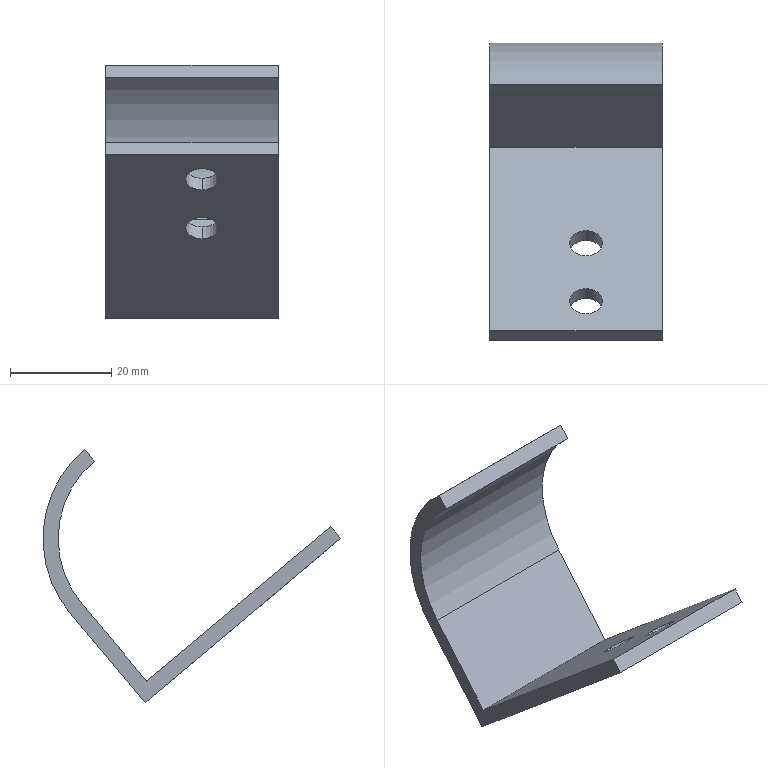Part | SolidWorks | features BaseBody 1 | 1 solid | 14 faces | box 34 x 58.835 x 50.022 mm | volume 10435 mm3 | plane 8 | cylinder 6 | commonest cylinder face diameters 6.5 x4 40 x1 46 x1
STEP:
#1=CARTESIAN_POINT('',(-85.,219.284,-334.482));
#2=VERTEX_POINT('',#1);
#3=CARTESIAN_POINT('',(-85.,224.263,-338.66));
#4=VERTEX_POINT('',#3);
#5=CARTESIAN_POINT('',(-85.,221.774,-336.571));
#6=DIRECTION('',(0.,-0.6428,-0.766));
#7=DIRECTION('',(0.,-0.766,0.6428));
#8=AXIS2_PLACEMENT_3D('',#5,#6,#7);
#9=CIRCLE('',#8,3.25);
#10=EDGE_CURVE('',#2,#4,#9,.T.);
#11=ORIENTED_EDGE('',*,*,#10,.T.);
#12=CARTESIAN_POINT('',(-85.,226.192,-336.362));
#13=VERTEX_POINT('',#12);
#14=CARTESIAN_POINT('',(-85.,219.764,-344.023));
#15=DIRECTION('',(0.,0.6428,0.766));
#16=VECTOR('',#15,1000.);
#17=LINE('',#14,#16);
#18=EDGE_CURVE('',#4,#13,#17,.T.);
#19=ORIENTED_EDGE('',*,*,#18,.T.);
#20=CARTESIAN_POINT('',(-85.,221.212,-332.184));
#21=VERTEX_POINT('',#20);
#22=CARTESIAN_POINT('',(-85.,223.702,-334.273));
#23=DIRECTION('',(0.,-0.6428,-0.766));
#24=DIRECTION('',(0.,-0.766,0.6428));
#25=AXIS2_PLACEMENT_3D('',#22,#23,#24);
#26=CIRCLE('',#25,3.25);
#27=EDGE_CURVE('',#21,#13,#26,.T.);
#28=ORIENTED_EDGE('',*,*,#27,.F.);
#29=CARTESIAN_POINT('',(-85.,214.785,-339.844));
#30=DIRECTION('',(0.,0.6428,0.766));
#31=VECTOR('',#30,1000.);
#32=LINE('',#29,#31);
#33=EDGE_CURVE('',#2,#21,#32,.T.);
#34=ORIENTED_EDGE('',*,*,#33,.F.);
#35=EDGE_LOOP('',(#11,#19,#28,#34));
#36=FACE_OUTER_BOUND('',#35,.T.);
#37=CARTESIAN_POINT('',(-85.,217.274,-341.934));
#38=DIRECTION('',(0.,0.6428,0.766));
#39=DIRECTION('',(0.,-0.766,0.6428));
#40=AXIS2_PLACEMENT_3D('',#37,#38,#39);
#41=CYLINDRICAL_SURFACE('',#40,3.25);
#42=ADVANCED_FACE('',(#36),#41,.F.);
#43=CARTESIAN_POINT('',(-85.,207.803,-324.848));
#44=VERTEX_POINT('',#43);
#45=CARTESIAN_POINT('',(-85.,212.782,-329.026));
#46=VERTEX_POINT('',#45);
#47=CARTESIAN_POINT('',(-85.,210.292,-326.937));
#48=DIRECTION('',(0.,-0.6428,-0.766));
#49=DIRECTION('',(0.,-0.766,0.6428));
#50=AXIS2_PLACEMENT_3D('',#47,#48,#49);
#51=CIRCLE('',#50,3.25);
#52=EDGE_CURVE('',#44,#46,#51,.T.);
#53=ORIENTED_EDGE('',*,*,#52,.T.);
#54=CARTESIAN_POINT('',(-85.,214.71,-326.728));
#55=VERTEX_POINT('',#54);
#56=CARTESIAN_POINT('',(-85.,208.282,-334.388));
#57=DIRECTION('',(0.,0.6428,0.766));
#58=VECTOR('',#57,1000.);
#59=LINE('',#56,#58);
#60=EDGE_CURVE('',#46,#55,#59,.T.);
#61=ORIENTED_EDGE('',*,*,#60,.T.);
#62=CARTESIAN_POINT('',(-85.,209.731,-322.55));
#63=VERTEX_POINT('',#62);
#64=CARTESIAN_POINT('',(-85.,212.221,-324.639));
#65=DIRECTION('',(0.,-0.6428,-0.766));
#66=DIRECTION('',(0.,-0.766,0.6428));
#67=AXIS2_PLACEMENT_3D('',#64,#65,#66);
#68=CIRCLE('',#67,3.25);
#69=EDGE_CURVE('',#63,#55,#68,.T.);
#70=ORIENTED_EDGE('',*,*,#69,.F.);
#71=CARTESIAN_POINT('',(-85.,203.303,-330.21));
#72=DIRECTION('',(0.,0.6428,0.766));
#73=VECTOR('',#72,1000.);
#74=LINE('',#71,#73);
#75=EDGE_CURVE('',#44,#63,#74,.T.);
#76=ORIENTED_EDGE('',*,*,#75,.F.);
#77=EDGE_LOOP('',(#53,#61,#70,#76));
#78=FACE_OUTER_BOUND('',#77,.T.);
#79=CARTESIAN_POINT('',(-85.,205.793,-332.299));
#80=DIRECTION('',(0.,0.6428,0.766));
#81=DIRECTION('',(0.,-0.766,0.6428));
#82=AXIS2_PLACEMENT_3D('',#79,#80,#81);
#83=CYLINDRICAL_SURFACE('',#82,3.25);
#84=ADVANCED_FACE('',(#78),#83,.F.);
#85=CARTESIAN_POINT('',(-104.,204.42,-322.01));
#86=VERTEX_POINT('',#85);
#87=CARTESIAN_POINT('',(-70.,204.42,-322.01));
#88=VERTEX_POINT('',#87);
#89=CARTESIAN_POINT('',(-100.,204.42,-322.01));
#90=DIRECTION('',(1.,0.,0.));
#91=VECTOR('',#90,1000.);
#92=LINE('',#89,#91);
#93=EDGE_CURVE('',#86,#88,#92,.T.);
#94=ORIENTED_EDGE('',*,*,#93,.F.);
#95=CARTESIAN_POINT('',(-104.,243.09,-354.458));
#96=VERTEX_POINT('',#95);
#97=CARTESIAN_POINT('',(-104.,243.09,-354.458));
#98=DIRECTION('',(0.,-0.766,0.6428));
#99=VECTOR('',#98,1000.);
#100=LINE('',#97,#99);
#101=EDGE_CURVE('',#96,#86,#100,.T.);
#102=ORIENTED_EDGE('',*,*,#101,.F.);
#103=CARTESIAN_POINT('',(-70.,243.09,-354.458));
#104=VERTEX_POINT('',#103);
#105=CARTESIAN_POINT('',(-100.,243.09,-354.458));
#106=DIRECTION('',(-1.,0.,0.));
#107=VECTOR('',#106,1000.);
#108=LINE('',#105,#107);
#109=EDGE_CURVE('',#104,#96,#108,.T.);
#110=ORIENTED_EDGE('',*,*,#109,.F.);
#111=CARTESIAN_POINT('',(-70.,243.09,-354.458));
#112=DIRECTION('',(0.,0.766,-0.6428));
#113=VECTOR('',#112,1000.);
#114=LINE('',#111,#113);
#115=EDGE_CURVE('',#88,#104,#114,.T.);
#116=ORIENTED_EDGE('',*,*,#115,.F.);
#117=EDGE_LOOP('',(#94,#102,#110,#116));
#118=FACE_OUTER_BOUND('',#117,.T.);
#119=ORIENTED_EDGE('',*,*,#10,.F.);
#120=CARTESIAN_POINT('',(-85.,221.774,-336.571));
#121=DIRECTION('',(0.,-0.6428,-0.766));
#122=DIRECTION('',(0.,-0.766,0.6428));
#123=AXIS2_PLACEMENT_3D('',#120,#121,#122);
#124=CIRCLE('',#123,3.25);
#125=EDGE_CURVE('',#4,#2,#124,.T.);
#126=ORIENTED_EDGE('',*,*,#125,.F.);
#127=EDGE_LOOP('',(#119,#126));
#128=FACE_BOUND('',#127,.T.);
#129=ORIENTED_EDGE('',*,*,#52,.F.);
#130=CARTESIAN_POINT('',(-85.,210.292,-326.937));
#131=DIRECTION('',(0.,-0.6428,-0.766));
#132=DIRECTION('',(0.,-0.766,0.6428));
#133=AXIS2_PLACEMENT_3D('',#130,#131,#132);
#134=CIRCLE('',#133,3.25);
#135=EDGE_CURVE('',#46,#44,#134,.T.);
#136=ORIENTED_EDGE('',*,*,#135,.F.);
#137=EDGE_LOOP('',(#129,#136));
#138=FACE_BOUND('',#137,.T.);
#139=CARTESIAN_POINT('',(-100.,243.09,-354.458));
#140=DIRECTION('',(0.,0.6428,0.766));
#141=DIRECTION('',(0.,-0.766,0.6428));
#142=AXIS2_PLACEMENT_3D('',#139,#140,#141);
#143=PLANE('',#142);
#144=ADVANCED_FACE('',(#118,#128,#138),#143,.F.);
#145=CARTESIAN_POINT('',(-70.,255.039,-304.436));
#146=VERTEX_POINT('',#145);
#147=CARTESIAN_POINT('',(-70.,253.111,-306.734));
#148=VERTEX_POINT('',#147);
#149=CARTESIAN_POINT('',(-70.,255.039,-304.436));
#150=DIRECTION('',(0.,-0.6428,-0.766));
#151=VECTOR('',#150,1000.);
#152=LINE('',#149,#151);
#153=EDGE_CURVE('',#146,#148,#152,.T.);
#154=ORIENTED_EDGE('',*,*,#153,.T.);
#155=CARTESIAN_POINT('',(-70.,255.576,-334.91));
#156=VERTEX_POINT('',#155);
#157=CARTESIAN_POINT('',(-70.,240.255,-322.055));
#158=DIRECTION('',(-1.,0.,0.));
#159=DIRECTION('',(0.,0.,-1.));
#160=AXIS2_PLACEMENT_3D('',#157,#158,#159);
#161=CIRCLE('',#160,20.);
#162=EDGE_CURVE('',#148,#156,#161,.T.);
#163=ORIENTED_EDGE('',*,*,#162,.T.);
#164=CARTESIAN_POINT('',(-70.,242.72,-350.231));
#165=VERTEX_POINT('',#164);
#166=CARTESIAN_POINT('',(-70.,255.576,-334.91));
#167=DIRECTION('',(0.,-0.6428,-0.766));
#168=VECTOR('',#167,1000.);
#169=LINE('',#166,#168);
#170=EDGE_CURVE('',#156,#165,#169,.T.);
#171=ORIENTED_EDGE('',*,*,#170,.T.);
#172=CARTESIAN_POINT('',(-70.,206.349,-319.712));
#173=VERTEX_POINT('',#172);
#174=CARTESIAN_POINT('',(-70.,242.72,-350.231));
#175=DIRECTION('',(0.,-0.766,0.6428));
#176=VECTOR('',#175,1000.);
#177=LINE('',#174,#176);
#178=EDGE_CURVE('',#165,#173,#177,.T.);
#179=ORIENTED_EDGE('',*,*,#178,.T.);
#180=CARTESIAN_POINT('',(-70.,206.349,-319.712));
#181=DIRECTION('',(0.,-0.6428,-0.766));
#182=VECTOR('',#181,1000.);
#183=LINE('',#180,#182);
#184=EDGE_CURVE('',#173,#88,#183,.T.);
#185=ORIENTED_EDGE('',*,*,#184,.T.);
#186=ORIENTED_EDGE('',*,*,#115,.T.);
#187=CARTESIAN_POINT('',(-70.,257.874,-336.839));
#188=VERTEX_POINT('',#187);
#189=CARTESIAN_POINT('',(-70.,243.09,-354.458));
#190=DIRECTION('',(0.,0.6428,0.766));
#191=VECTOR('',#190,1000.);
#192=LINE('',#189,#191);
#193=EDGE_CURVE('',#104,#188,#192,.T.);
#194=ORIENTED_EDGE('',*,*,#193,.T.);
#195=CARTESIAN_POINT('',(-70.,240.255,-322.055));
#196=DIRECTION('',(1.,0.,0.));
#197=DIRECTION('',(0.,0.,-1.));
#198=AXIS2_PLACEMENT_3D('',#195,#196,#197);
#199=CIRCLE('',#198,23.);
#200=EDGE_CURVE('',#188,#146,#199,.T.);
#201=ORIENTED_EDGE('',*,*,#200,.T.);
#202=EDGE_LOOP('',(#154,#163,#171,#179,#185,#186,#194,#201));
#203=FACE_OUTER_BOUND('',#202,.T.);
#204=CARTESIAN_POINT('',(-70.,240.255,-322.055));
#205=DIRECTION('',(1.,0.,0.));
#206=DIRECTION('',(0.,0.,-1.));
#207=AXIS2_PLACEMENT_3D('',#204,#205,#206);
#208=PLANE('',#207);
#209=ADVANCED_FACE('',(#203),#208,.T.);
#210=CARTESIAN_POINT('',(-104.,206.349,-319.712));
#211=VERTEX_POINT('',#210);
#212=CARTESIAN_POINT('',(-100.,206.349,-319.712));
#213=DIRECTION('',(1.,0.,0.));
#214=VECTOR('',#213,1000.);
#215=LINE('',#212,#214);
#216=EDGE_CURVE('',#211,#173,#215,.T.);
#217=ORIENTED_EDGE('',*,*,#216,.F.);
#218=CARTESIAN_POINT('',(-104.,206.349,-319.712));
#219=DIRECTION('',(0.,0.6428,0.766));
#220=VECTOR('',#219,1000.);
#221=LINE('',#218,#220);
#222=EDGE_CURVE('',#86,#211,#221,.T.);
#223=ORIENTED_EDGE('',*,*,#222,.F.);
#224=ORIENTED_EDGE('',*,*,#93,.T.);
#225=ORIENTED_EDGE('',*,*,#184,.F.);
#226=EDGE_LOOP('',(#217,#223,#224,#225));
#227=FACE_OUTER_BOUND('',#226,.T.);
#228=CARTESIAN_POINT('',(-100.,206.349,-319.712));
#229=DIRECTION('',(0.,0.766,-0.6428));
#230=DIRECTION('',(0.,0.6428,0.766));
#231=AXIS2_PLACEMENT_3D('',#228,#229,#230);
#232=PLANE('',#231);
#233=ADVANCED_FACE('',(#227),#232,.F.);
#234=CARTESIAN_POINT('',(-104.,253.111,-306.734));
#235=VERTEX_POINT('',#234);
#236=CARTESIAN_POINT('',(-104.,255.576,-334.91));
#237=VERTEX_POINT('',#236);
#238=CARTESIAN_POINT('',(-104.,240.255,-322.055));
#239=DIRECTION('',(-1.,0.,0.));
#240=DIRECTION('',(0.,0.,-1.));
#241=AXIS2_PLACEMENT_3D('',#238,#239,#240);
#242=CIRCLE('',#241,20.);
#243=EDGE_CURVE('',#235,#237,#242,.T.);
#244=ORIENTED_EDGE('',*,*,#243,.F.);
#245=CARTESIAN_POINT('',(-104.,255.039,-304.436));
#246=VERTEX_POINT('',#245);
#247=CARTESIAN_POINT('',(-104.,255.039,-304.436));
#248=DIRECTION('',(0.,-0.6428,-0.766));
#249=VECTOR('',#248,1000.);
#250=LINE('',#247,#249);
#251=EDGE_CURVE('',#246,#235,#250,.T.);
#252=ORIENTED_EDGE('',*,*,#251,.F.);
#253=CARTESIAN_POINT('',(-104.,257.874,-336.839));
#254=VERTEX_POINT('',#253);
#255=CARTESIAN_POINT('',(-104.,240.255,-322.055));
#256=DIRECTION('',(1.,0.,0.));
#257=DIRECTION('',(0.,0.,-1.));
#258=AXIS2_PLACEMENT_3D('',#255,#256,#257);
#259=CIRCLE('',#258,23.);
#260=EDGE_CURVE('',#254,#246,#259,.T.);
#261=ORIENTED_EDGE('',*,*,#260,.F.);
#262=CARTESIAN_POINT('',(-104.,243.09,-354.458));
#263=DIRECTION('',(0.,0.6428,0.766));
#264=VECTOR('',#263,1000.);
#265=LINE('',#262,#264);
#266=EDGE_CURVE('',#96,#254,#265,.T.);
#267=ORIENTED_EDGE('',*,*,#266,.F.);
#268=ORIENTED_EDGE('',*,*,#101,.T.);
#269=ORIENTED_EDGE('',*,*,#222,.T.);
#270=CARTESIAN_POINT('',(-104.,242.72,-350.231));
#271=VERTEX_POINT('',#270);
#272=CARTESIAN_POINT('',(-104.,242.72,-350.231));
#273=DIRECTION('',(0.,-0.766,0.6428));
#274=VECTOR('',#273,1000.);
#275=LINE('',#272,#274);
#276=EDGE_CURVE('',#271,#211,#275,.T.);
#277=ORIENTED_EDGE('',*,*,#276,.F.);
#278=CARTESIAN_POINT('',(-104.,255.576,-334.91));
#279=DIRECTION('',(0.,-0.6428,-0.766));
#280=VECTOR('',#279,1000.);
#281=LINE('',#278,#280);
#282=EDGE_CURVE('',#237,#271,#281,.T.);
#283=ORIENTED_EDGE('',*,*,#282,.F.);
#284=EDGE_LOOP('',(#244,#252,#261,#267,#268,#269,#277,#283));
#285=FACE_OUTER_BOUND('',#284,.T.);
#286=CARTESIAN_POINT('',(-104.,240.255,-322.055));
#287=DIRECTION('',(1.,0.,0.));
#288=DIRECTION('',(0.,0.,-1.));
#289=AXIS2_PLACEMENT_3D('',#286,#287,#288);
#290=PLANE('',#289);
#291=ADVANCED_FACE('',(#285),#290,.F.);
#292=ORIENTED_EDGE('',*,*,#109,.T.);
#293=ORIENTED_EDGE('',*,*,#266,.T.);
#294=CARTESIAN_POINT('',(-100.,257.874,-336.839));
#295=DIRECTION('',(-1.,0.,0.));
#296=VECTOR('',#295,1000.);
#297=LINE('',#294,#296);
#298=EDGE_CURVE('',#188,#254,#297,.T.);
#299=ORIENTED_EDGE('',*,*,#298,.F.);
#300=ORIENTED_EDGE('',*,*,#193,.F.);
#301=EDGE_LOOP('',(#292,#293,#299,#300));
#302=FACE_OUTER_BOUND('',#301,.T.);
#303=CARTESIAN_POINT('',(-100.,243.09,-354.458));
#304=DIRECTION('',(0.,-0.766,0.6428));
#305=DIRECTION('',(0.,-0.6428,-0.766));
#306=AXIS2_PLACEMENT_3D('',#303,#304,#305);
#307=PLANE('',#306);
#308=ADVANCED_FACE('',(#302),#307,.F.);
#309=ORIENTED_EDGE('',*,*,#18,.F.);
#310=ORIENTED_EDGE('',*,*,#125,.T.);
#311=ORIENTED_EDGE('',*,*,#33,.T.);
#312=CARTESIAN_POINT('',(-85.,223.702,-334.273));
#313=DIRECTION('',(0.,-0.6428,-0.766));
#314=DIRECTION('',(0.,-0.766,0.6428));
#315=AXIS2_PLACEMENT_3D('',#312,#313,#314);
#316=CIRCLE('',#315,3.25);
#317=EDGE_CURVE('',#13,#21,#316,.T.);
#318=ORIENTED_EDGE('',*,*,#317,.F.);
#319=EDGE_LOOP('',(#309,#310,#311,#318));
#320=FACE_OUTER_BOUND('',#319,.T.);
#321=CARTESIAN_POINT('',(-85.,217.274,-341.934));
#322=DIRECTION('',(0.,0.6428,0.766));
#323=DIRECTION('',(0.,-0.766,0.6428));
#324=AXIS2_PLACEMENT_3D('',#321,#322,#323);
#325=CYLINDRICAL_SURFACE('',#324,3.25);
#326=ADVANCED_FACE('',(#320),#325,.F.);
#327=ORIENTED_EDGE('',*,*,#60,.F.);
#328=ORIENTED_EDGE('',*,*,#135,.T.);
#329=ORIENTED_EDGE('',*,*,#75,.T.);
#330=CARTESIAN_POINT('',(-85.,212.221,-324.639));
#331=DIRECTION('',(0.,-0.6428,-0.766));
#332=DIRECTION('',(0.,-0.766,0.6428));
#333=AXIS2_PLACEMENT_3D('',#330,#331,#332);
#334=CIRCLE('',#333,3.25);
#335=EDGE_CURVE('',#55,#63,#334,.T.);
#336=ORIENTED_EDGE('',*,*,#335,.F.);
#337=EDGE_LOOP('',(#327,#328,#329,#336));
#338=FACE_OUTER_BOUND('',#337,.T.);
#339=CARTESIAN_POINT('',(-85.,205.793,-332.299));
#340=DIRECTION('',(0.,0.6428,0.766));
#341=DIRECTION('',(0.,-0.766,0.6428));
#342=AXIS2_PLACEMENT_3D('',#339,#340,#341);
#343=CYLINDRICAL_SURFACE('',#342,3.25);
#344=ADVANCED_FACE('',(#338),#343,.F.);
#345=CARTESIAN_POINT('',(-100.,253.111,-306.734));
#346=DIRECTION('',(1.,0.,0.));
#347=VECTOR('',#346,1000.);
#348=LINE('',#345,#347);
#349=EDGE_CURVE('',#235,#148,#348,.T.);
#350=ORIENTED_EDGE('',*,*,#349,.F.);
#351=ORIENTED_EDGE('',*,*,#243,.T.);
#352=CARTESIAN_POINT('',(-100.,255.576,-334.91));
#353=DIRECTION('',(-1.,0.,0.));
#354=VECTOR('',#353,1000.);
#355=LINE('',#352,#354);
#356=EDGE_CURVE('',#156,#237,#355,.T.);
#357=ORIENTED_EDGE('',*,*,#356,.F.);
#358=ORIENTED_EDGE('',*,*,#162,.F.);
#359=EDGE_LOOP('',(#350,#351,#357,#358));
#360=FACE_OUTER_BOUND('',#359,.T.);
#361=CARTESIAN_POINT('',(-100.,240.255,-322.055));
#362=DIRECTION('',(1.,0.,0.));
#363=DIRECTION('',(0.,0.,-1.));
#364=AXIS2_PLACEMENT_3D('',#361,#362,#363);
#365=CYLINDRICAL_SURFACE('',#364,20.);
#366=ADVANCED_FACE('',(#360),#365,.F.);
#367=CARTESIAN_POINT('',(-100.,255.039,-304.436));
#368=DIRECTION('',(1.,0.,0.));
#369=VECTOR('',#368,1000.);
#370=LINE('',#367,#369);
#371=EDGE_CURVE('',#246,#146,#370,.T.);
#372=ORIENTED_EDGE('',*,*,#371,.F.);
#373=ORIENTED_EDGE('',*,*,#251,.T.);
#374=ORIENTED_EDGE('',*,*,#349,.T.);
#375=ORIENTED_EDGE('',*,*,#153,.F.);
#376=EDGE_LOOP('',(#372,#373,#374,#375));
#377=FACE_OUTER_BOUND('',#376,.T.);
#378=CARTESIAN_POINT('',(-100.,253.111,-306.734));
#379=DIRECTION('',(0.,0.766,-0.6428));
#380=DIRECTION('',(0.,0.6428,0.766));
#381=AXIS2_PLACEMENT_3D('',#378,#379,#380);
#382=PLANE('',#381);
#383=ADVANCED_FACE('',(#377),#382,.F.);
#384=ORIENTED_EDGE('',*,*,#260,.T.);
#385=ORIENTED_EDGE('',*,*,#371,.T.);
#386=ORIENTED_EDGE('',*,*,#200,.F.);
#387=ORIENTED_EDGE('',*,*,#298,.T.);
#388=EDGE_LOOP('',(#384,#385,#386,#387));
#389=FACE_OUTER_BOUND('',#388,.T.);
#390=CARTESIAN_POINT('',(-100.,240.255,-322.055));
#391=DIRECTION('',(1.,0.,0.));
#392=DIRECTION('',(0.,0.,-1.));
#393=AXIS2_PLACEMENT_3D('',#390,#391,#392);
#394=CYLINDRICAL_SURFACE('',#393,23.);
#395=ADVANCED_FACE('',(#389),#394,.T.);
#396=CARTESIAN_POINT('',(-100.,242.72,-350.231));
#397=DIRECTION('',(1.,0.,0.));
#398=VECTOR('',#397,1000.);
#399=LINE('',#396,#398);
#400=EDGE_CURVE('',#271,#165,#399,.T.);
#401=ORIENTED_EDGE('',*,*,#400,.F.);
#402=ORIENTED_EDGE('',*,*,#276,.T.);
#403=ORIENTED_EDGE('',*,*,#216,.T.);
#404=ORIENTED_EDGE('',*,*,#178,.F.);
#405=EDGE_LOOP('',(#401,#402,#403,#404));
#406=FACE_OUTER_BOUND('',#405,.T.);
#407=ORIENTED_EDGE('',*,*,#27,.T.);
#408=ORIENTED_EDGE('',*,*,#317,.T.);
#409=EDGE_LOOP('',(#407,#408));
#410=FACE_BOUND('',#409,.T.);
#411=ORIENTED_EDGE('',*,*,#69,.T.);
#412=ORIENTED_EDGE('',*,*,#335,.T.);
#413=EDGE_LOOP('',(#411,#412));
#414=FACE_BOUND('',#413,.T.);
#415=CARTESIAN_POINT('',(-100.,242.72,-350.231));
#416=DIRECTION('',(0.,-0.6428,-0.766));
#417=DIRECTION('',(0.,0.766,-0.6428));
#418=AXIS2_PLACEMENT_3D('',#415,#416,#417);
#419=PLANE('',#418);
#420=ADVANCED_FACE('',(#406,#410,#414),#419,.F.);
#421=ORIENTED_EDGE('',*,*,#356,.T.);
#422=ORIENTED_EDGE('',*,*,#282,.T.);
#423=ORIENTED_EDGE('',*,*,#400,.T.);
#424=ORIENTED_EDGE('',*,*,#170,.F.);
#425=EDGE_LOOP('',(#421,#422,#423,#424));
#426=FACE_OUTER_BOUND('',#425,.T.);
#427=CARTESIAN_POINT('',(-100.,242.72,-350.231));
#428=DIRECTION('',(0.,0.766,-0.6428));
#429=DIRECTION('',(0.,0.6428,0.766));
#430=AXIS2_PLACEMENT_3D('',#427,#428,#429);
#431=PLANE('',#430);
#432=ADVANCED_FACE('',(#426),#431,.F.);
#433=CLOSED_SHELL('',(#42,#84,#144,#209,#233,#291,#308,#326,#344,#366,#383,#395,#420,#432));
#434=MANIFOLD_SOLID_BREP('',#433);
#435=CARTESIAN_POINT('',(0.,0.,0.));
#436=DIRECTION('',(0.,0.,1.));
#437=DIRECTION('',(1.,0.,0.));
#438=AXIS2_PLACEMENT_3D('',#435,#436,#437);
#439=(LENGTH_UNIT()NAMED_UNIT(*)SI_UNIT(.MILLI.,.METRE.));
#440=UNCERTAINTY_MEASURE_WITH_UNIT(LENGTH_MEASURE(0.00001),#439,'','');
#441=(NAMED_UNIT(*)PLANE_ANGLE_UNIT()SI_UNIT($,.RADIAN.));
#442=(NAMED_UNIT(*)SI_UNIT($,.STERADIAN.)SOLID_ANGLE_UNIT());
#443=(GEOMETRIC_REPRESENTATION_CONTEXT(3)GLOBAL_UNCERTAINTY_ASSIGNED_CONTEXT((#440))GLOBAL_UNIT_ASSIGNED_CONTEXT((#439,#441,#442))REPRESENTATION_CONTEXT('',''));
#444=ADVANCED_BREP_SHAPE_REPRESENTATION('',(#434,#438),#443);